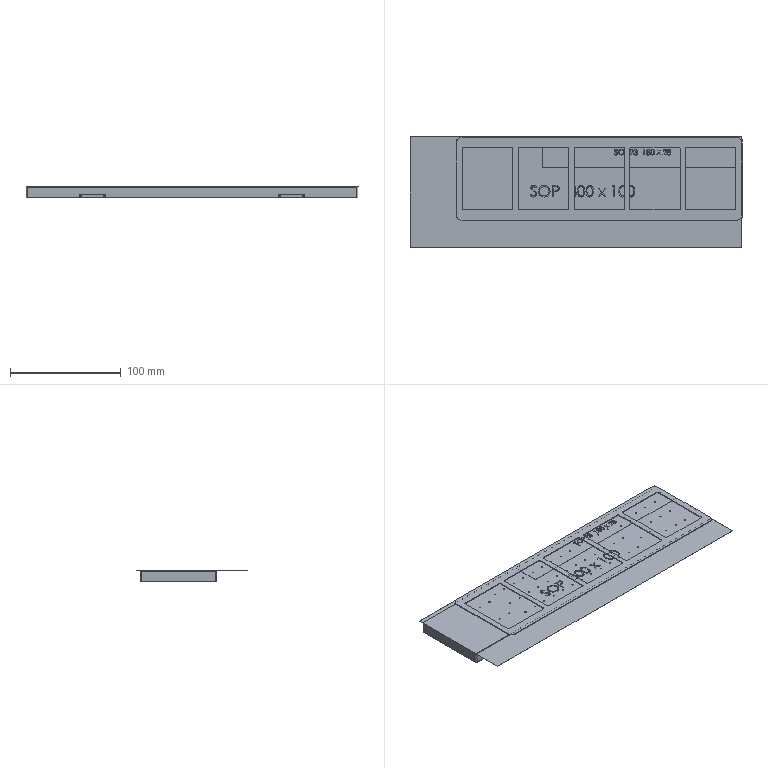Part | NX | features BREP 19 | 22 solids | 876 faces | box 300 x 100 x 10.8 mm | volume 198178 mm3 | cylinder 358 | plane 254 | spline 174 | cone 90 | commonest cylinder face diameters 4 x180 1 x112 2 x28 2.5 x8 3.4 x8 7 x8